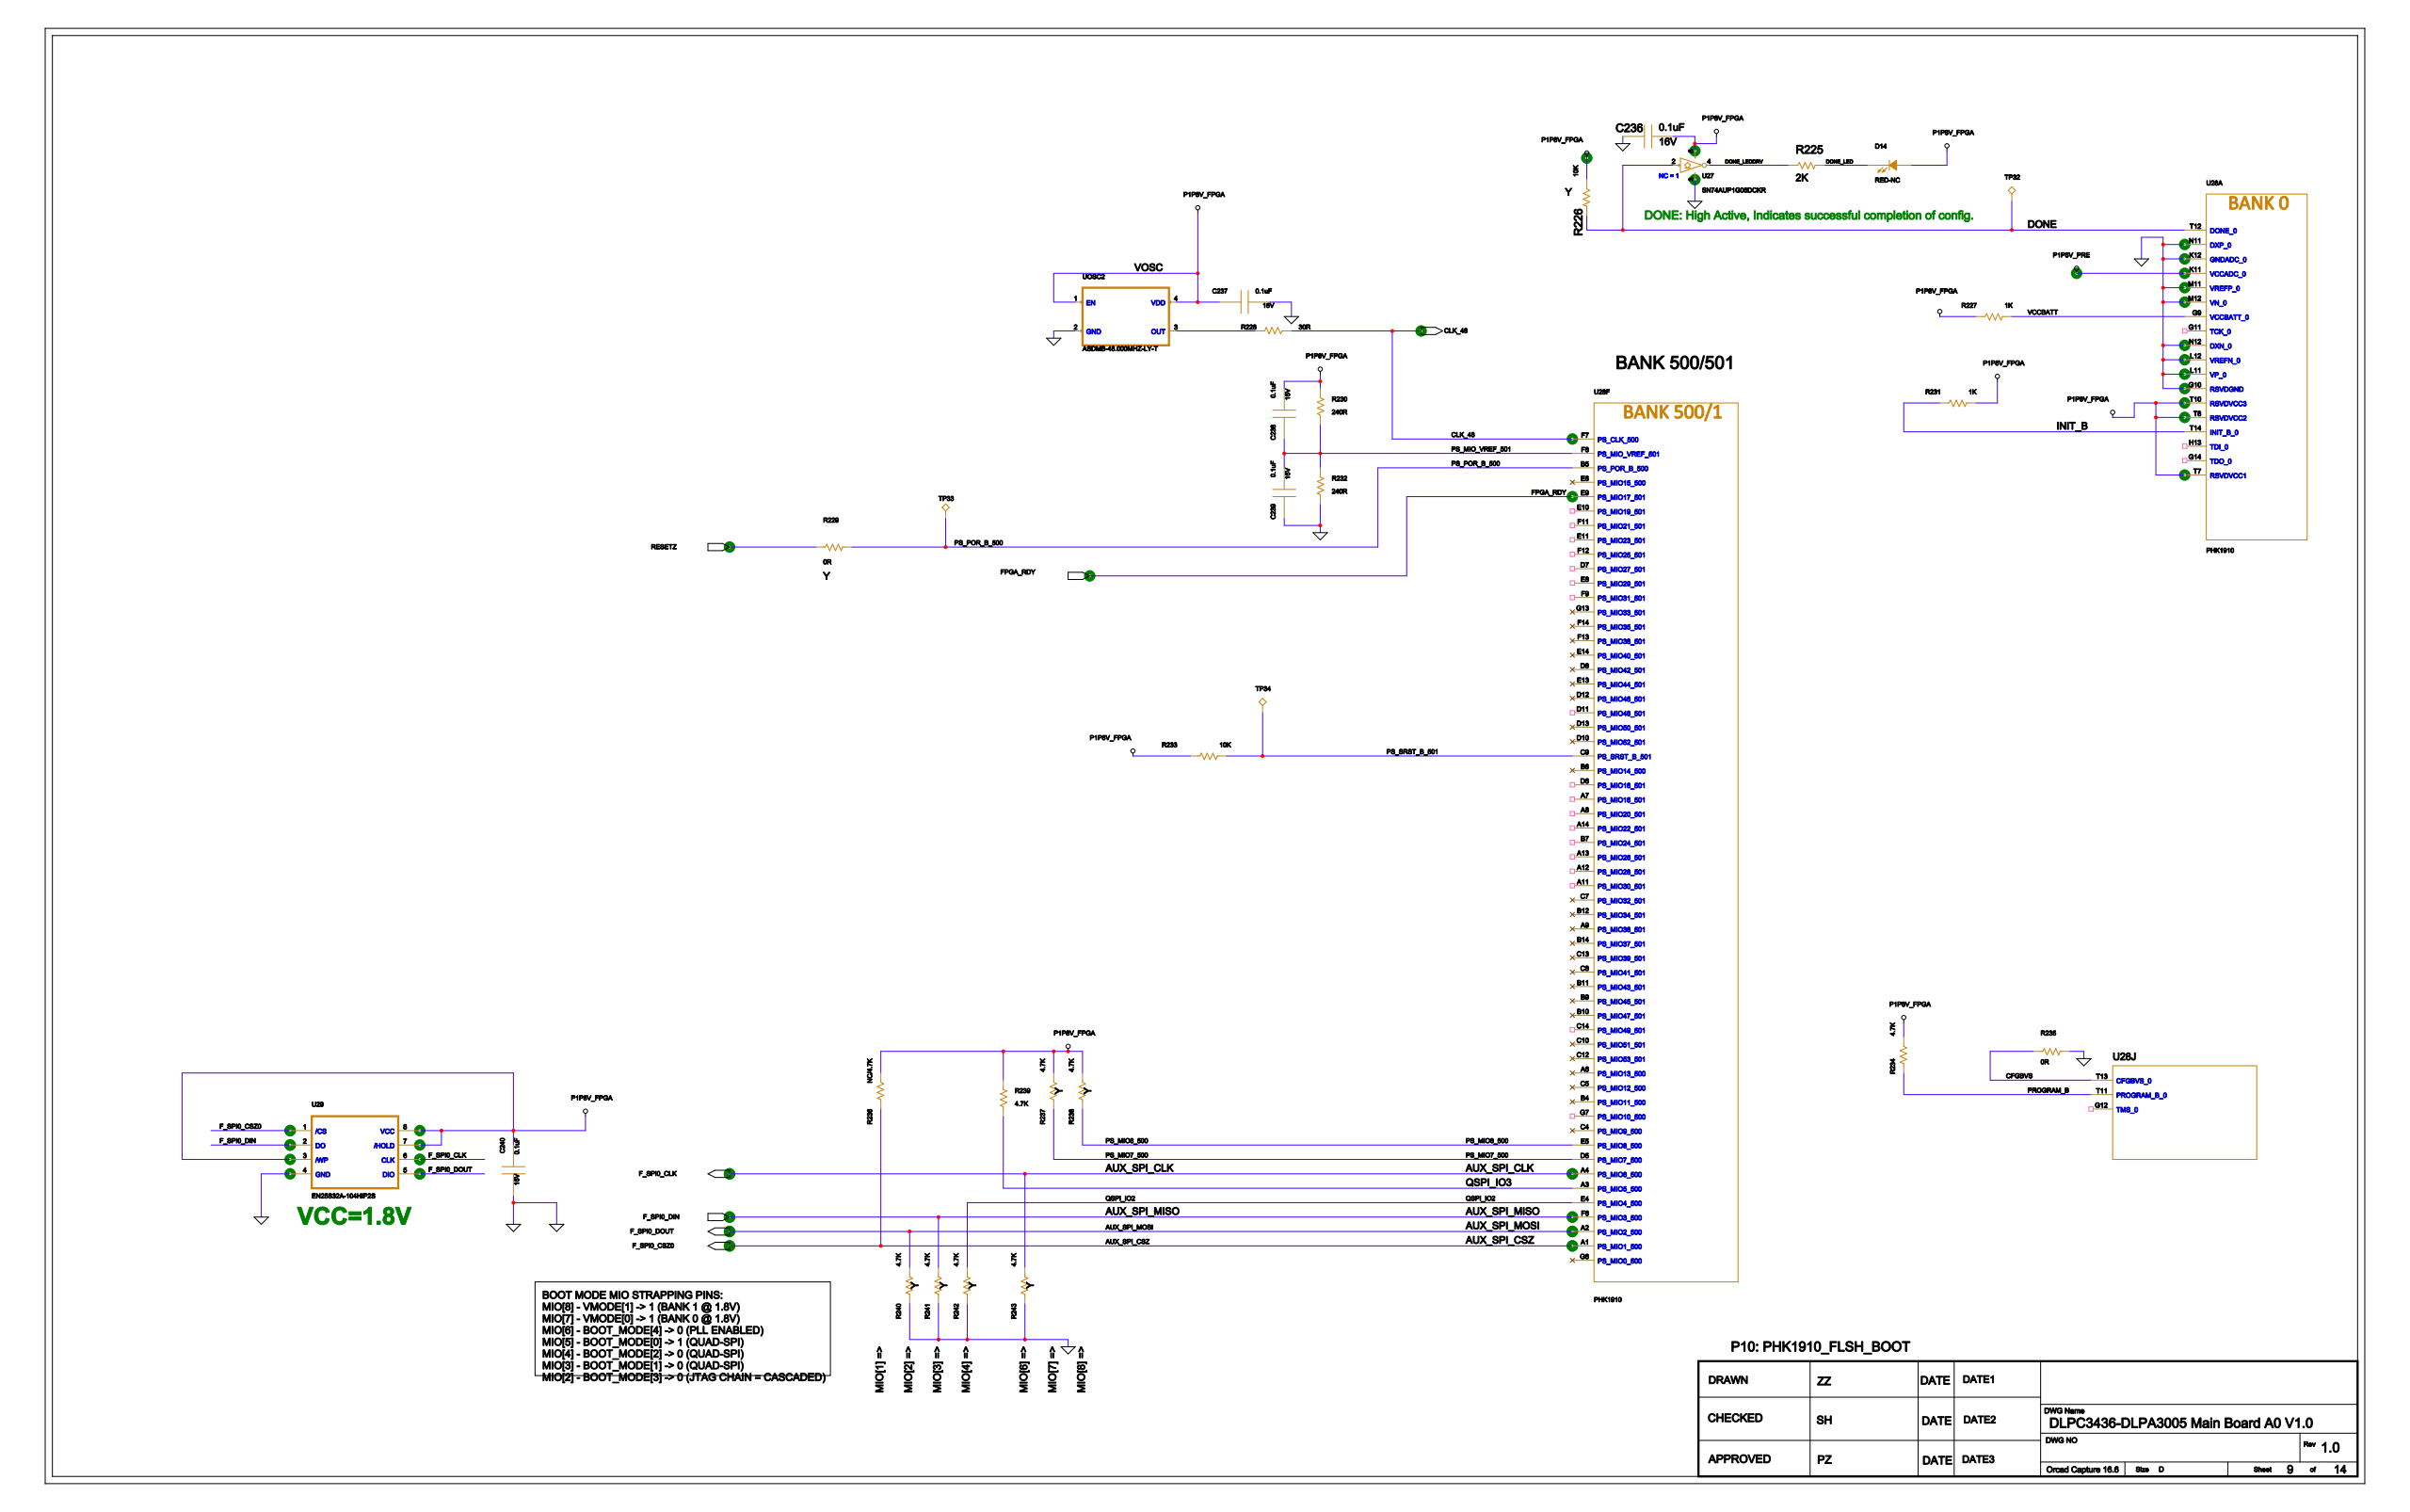Circuit board | Cadence Allegro | 1223 parts | 777 nets | one sheet of the schematic
Parts on this sheet (reference | value | footprint):
C236 | 0.1uF | C0201
C237 | 0.1uF | C0201
C238 | 0.1uF | C0201
C239 | 0.1uF | C0201
C240 | 0.1uF | C0201
D14 | RED-NC | SMD-LED
R225 | 2K | R0201
R226 | 10K | R0201
R227 | 1K | R0201
R228 | 30R | R0201
R229 | 0R | R0201
R230 | 240R | R0402
R231 | 1K | R0201
R232 | 240R | R0402
R233 | 10K | R0201
R234 | 4.7K | R0201
R235 | 0R | R0402
R236 | NC/4.7K | R0201
R237 | 4.7K | R0201
R238 | 4.7K | R0201
R239 | 4.7K | R0201
R240 | 4.7K | R0201
R241 | 4.7K | R0201
R242 | 4.7K | R0201
R243 | 4.7K | R0201
TP32 | TP40 | TP06MM
TP33 | TP40 | TP06MM
TP34 | TP40 | TP06MM
U27 | SN74AUP1G06DCK | U_5_DCK
U28 | PHK1910 | XILINX_CLG484
U29 | EN25S32A-104HIP2S | SOIC-8_208MIL
UOSC2 | 48MHz | CRY-D3225
Nets of these parts (net: part-pin ...):
GND: C236-1 C237-2 C239-2 C240-2 R232-2 R235-1 R240-1 R241-1 R242-1 R243-1 U27-3 U29-4 UOSC2-2 U28-D14 U28-G10 U28-K12 U28-L11 U28-L12 U28-M11 U28-M12 U28-N11 U28-N12 U28-P10
P1P8V_PRE: U28-K11
P1P8V_FPGA: C236-2 C237-1 C238-1 C240-1 D14-1 R226-2 R227-2 R230-1 R231-1 R233-2 R234-2 R236-2 R237-2 R238-2 R239-1 U27-5 U29-3 U29-7 U29-8 UOSC2-1 UOSC2-4 U28-T7 U28-T8 U28-T10
PS_MIO_VREF_501: C238-2 C239-1 R230-2 R232-1 U28-F8
DONE_LED: D14-2 R225-1
DONE: R226-1 TP32-1 U27-2 U28-T12
PS_POR_B_500: R229-1 TP33-1 U28-B5
PS_SRST_B_501: R233-1 TP34-1 U28-C9
RESETZ: R229-2
N22206907: R228-1 UOSC2-3
CLK_48: R228-2 U28-F7
DONE_LEDDRV: R225-2 U27-4
FPGA_RDY: U28-E9
VCCBATT: R227-1 U28-G9
INIT_B: R231-2 U28-T14
PROGRAM_B: R234-1 U28-T11
PS_MIO7_500: R237-1 U28-D5
PS_MIO8_500: R238-1 U28-E5
QSPI_IO3: R239-2 U28-A3
F_SPI0_DOUT: R240-2 U29-5 U28-A2
F_SPI0_DIN: R241-2 U29-2 U28-F6
QSPI_IO2: R242-2 U28-E4
F_SPI0_CLK: R243-2 U29-6 U28-A4
CFGBVS: R235-2 U28-T13
F_SPI0_CSZ0: R236-1 U29-1 U28-A1